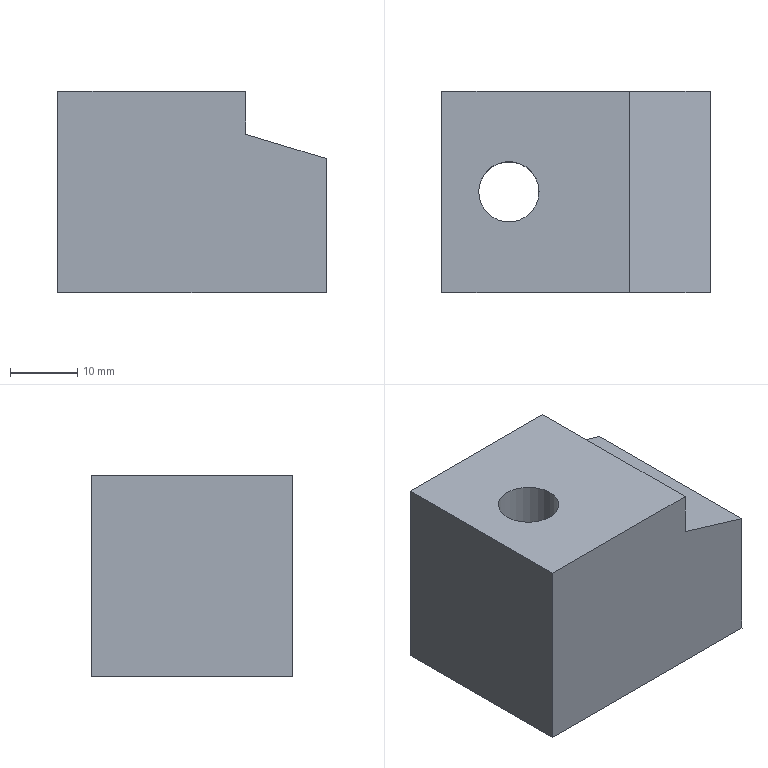Part | STEP file | solid 20 | 1 solid | 11 faces | box 40 x 30 x 30 mm | volume 30325 mm3 | plane 9 | cylinder 2 | commonest cylinder face diameters 9 x1 14 x1